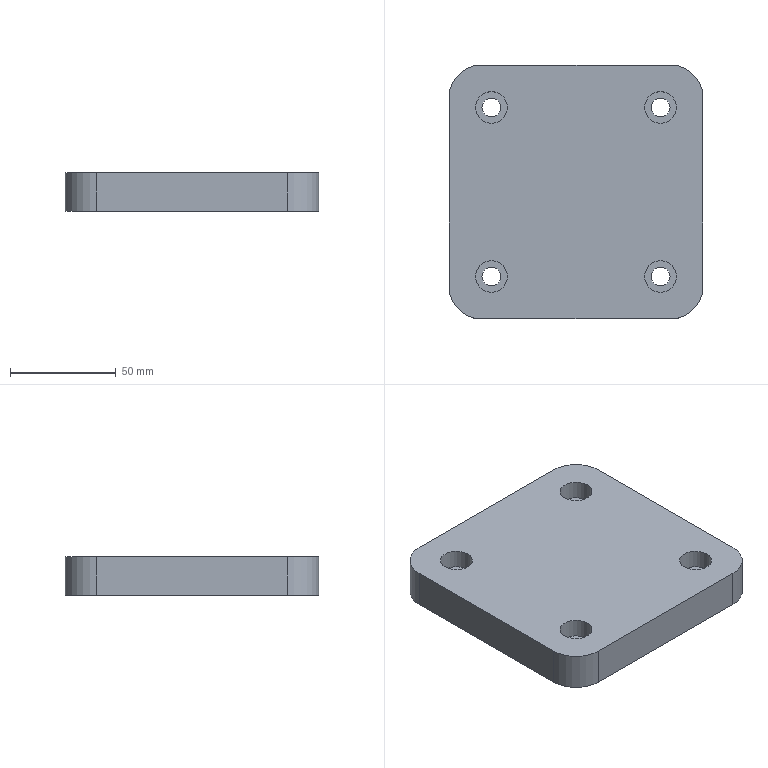Part | STEP file | solid 51 | 1 solid | 22 faces | box 120 x 120 x 18 mm | volume 247072 mm3 | cylinder 12 | plane 10 | commonest cylinder face diameters 9 x4 15 x4 30 x4